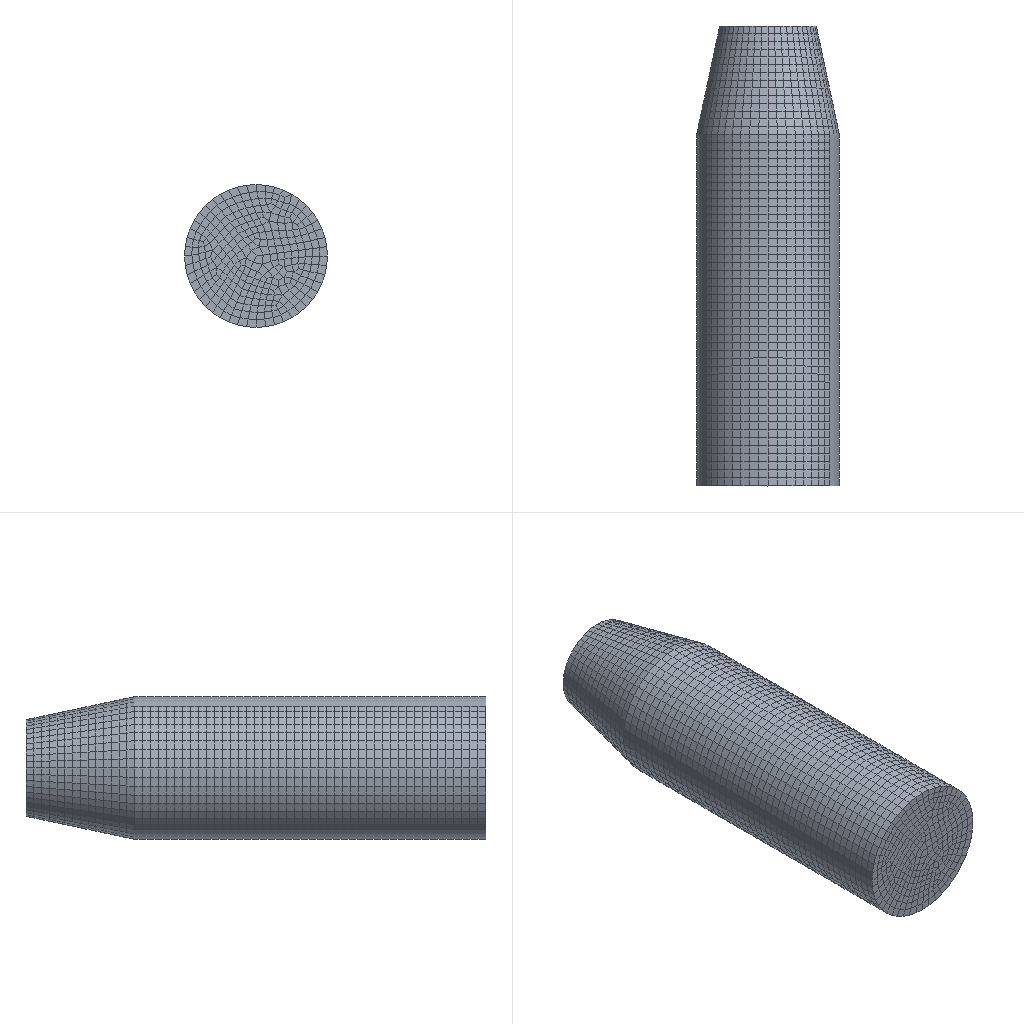Simulation study | abaqus
Set-up summary:
category,name,step,type,value,unit,region
solver,abaqus
solver,version,,,Abaqus/Explicit 3DEXPERIENCE R2017x
units,not stated in the deck,,not stated
analysis,deck,,transient,transient
load_step,Step-1,Step-1,transient
load_step,requested,,,1
mesh,nodes,,,20181
mesh,elements,,,18386
element_type,C3D8RT,,solid,18386
load,load commands in deck,,count,4
bc,support commands in deck,,count,20
material,MATERIAL-2,,in results
material,ZHAJIAN,,in results
check,setup vs results,,match,"per instance, exact: element labels, types and connectivity; labels of the nodes the elements use; coordinates of those nodes at SINGLE_PRECISION in 3 of 4 instance(s)"
Abaqus input file, long lists of numbers shortened:
*Heading
** Job name: Job-7 Model name: Job-model-Copy
** Generated by: Abaqus/CAE 2017
*Preprint, echo=NO, model=NO, history=NO, contact=NO
**
** PARTS
**
*Part, name=GUN-1
*End Part
**
*Part, name=GUN-2
*End Part
**
*Part, name=GUN-3
*End Part
**
*Part, name=ZHAJIAN
*Node
      1,        16.25,           0.,           0.
      2,           0.,           0.,           0.
** (20176 more lines like these left out)
*Element, type=C3D8RT
    1,   436,   447,   424,   454,    94,   105,    82,   112
    2,   379,   447,   436,   378,    37,   105,    94,    36
** (18384 more lines like these left out)
*Nset, nset=SET-1, generate
     1,  20178,      1
*Elset, elset=SET-1, generate
     1,  18386,      1
*Nset, nset=SET-16, generate
     1,  20178,      1
*Elset, elset=SET-16, generate
     1,  18386,      1
*Nset, nset=SET-17, generate
     1,  20178,      1
*Elset, elset=SET-17, generate
     1,  18386,      1
*Nset, nset=SET-21, generate
     1,  20178,      1
*Elset, elset=SET-21, generate
     1,  18386,      1
*Nset, nset=SET-22, generate
     1,  20178,      1
*Elset, elset=SET-22, generate
     1,  18386,      1
*Nset, nset=SET-23, generate
     1,  20178,      1
*Elset, elset=SET-23, generate
     1,  18386,      1
*Nset, nset=SET-24, generate
     1,  20178,      1
*Elset, elset=SET-24, generate
     1,  18386,      1
*Nset, nset=SET-25, generate
     1,  20178,      1
*Elset, elset=SET-25, generate
     1,  18386,      1
*Nset, nset=SET-26, generate
     1,  20178,      1
*Elset, elset=SET-26, generate
     1,  18386,      1
*Nset, nset=SET-27, generate
     1,  20178,      1
*Elset, elset=SET-27, generate
     1,  18386,      1
*Nset, nset=SET-28, generate
     1,  20178,      1
*Elset, elset=SET-28, generate
     1,  18386,      1
*Nset, nset=SET-29, generate
     1,  20178,      1
*Elset, elset=SET-29, generate
     1,  18386,      1
*Nset, nset=SET-30, generate
     1,  20178,      1
*Elset, elset=SET-30, generate
     1,  18386,      1
** Section: Section-1-SET-30
*Solid Section, elset=SET-30, material=ZHAJIAN
,
*End Part
**
**
** ASSEMBLY
**
*Assembly, name=Assembly
**
*Instance, name=GUN-1, part=GUN-1
-55.131,         110., -14.51
-55.131,         110., -14.51, -54.742, 109.611, -13.675, 159.423
*Node
      1,           0.,           0.,  -3.36777865e-15
*Nset, nset=GUN-1-RefPt_, internal
 1,
*Nset, nset=GUN-1-REFPT_, internal
 1,
*Surface, type=REVOLUTION, name=GUN-1-M_SURF-21
START,          55.,           0.
 LINE, 33.911, -30.343
 CIRCL, 31.217, -33.682, 9.277, -13.222
 LINE, 17.483, -48.41
 CIRCL, 13.826,         -50., 13.826,         -45.
 LINE,          10.,         -50.
*End Instance
**
*Instance, name=ZHAJIAN-1, part=ZHAJIAN
          0.,           0.,           0.
          0.,           0.,           0.,           0.,          -1.,           0., 7.5
*End Instance
**
*Instance, name=GUN-2, part=GUN-2
40.131,         110., -40.49
40.131,         110., -40.49, 39.596, 109.643, -39.725, 208.057
*Node
      1,           0.,           0.,  -3.36777865e-15
*Nset, nset=GUN-2-RefPt_, internal
 1,
*Nset, nset=GUN-2-REFPT_, internal
 1,
*Surface, type=REVOLUTION, name=GUN-2-M_SURF-19
START,          55.,           0.
 LINE, 33.911, -30.343
 CIRCL, 31.217, -33.682, 9.277, -13.222
 LINE, 17.483, -48.41
 CIRCL, 13.826,         -50., 13.826,         -45.
 LINE,          10.,         -50.
*End Instance
**
*Instance, name=GUN-3, part=GUN-3
         15.,         110.,          55.
         15.,         110.,          55., 15.995, 109.959, 55.087, 130.203
*Node
      1,           0.,           0.,  -3.36777865e-15
*Nset, nset=GUN-3-RefPt_, internal
 1,
*Nset, nset=GUN-3-REFPT_, internal
 1,
*Surface, type=REVOLUTION, name=GUN-3-M_SURF-27
START,          55.,           0.
 LINE, 33.911, -30.343
 CIRCL, 31.217, -33.682, 9.277, -13.222
 LINE, 17.483, -48.41
 CIRCL, 13.826,         -50., 13.826,         -45.
 LINE,          10.,         -50.
*End Instance
**
*Node
      1,           0.,    104.699,           0.
      2,           0.,           0.,           0.
*Nset, nset=M_SET-28
 1,
*Nset, nset=M_SET-42
 2,
*Nset, nset=M_SET-43
 1,
*Nset, nset=SET-30, instance=GUN-1
 1,
*Nset, nset=SET-30, instance=GUN-2
 1,
*Nset, nset=SET-31, instance=GUN-1
 1,
*Nset, nset=SET-32, instance=GUN-2
 1,
*Nset, nset=SET-34
 1,
*Nset, nset=SET-35, instance=ZHAJIAN-1, generate
     1,  20178,      1
*Elset, elset=SET-35, instance=ZHAJIAN-1, generate
     1,  18386,      1
*Nset, nset=SET-36, instance=GUN-2
 1,
*Nset, nset=SET-38, instance=GUN-1
 1,
*Nset, nset=SET-38, instance=GUN-2
 1,
*Nset, nset=SET-38, instance=GUN-3
 1,
*Nset, nset=SET-39, instance=GUN-3
 1,
*Nset, nset=SET-44
 1, 2
*Nset, nset=SET-45, instance=ZHAJIAN-1, generate
     1,  20178,      1
*Nset, nset=SET-45
 2,
*Elset, elset=SET-45, instance=ZHAJIAN-1, generate
     1,  18386,      1
*Nset, nset=SET-46, instance=GUN-2
 1,
*Nset, nset=SET-47, instance=GUN-1
 1,
*Nset, nset=SET-48, instance=GUN-2
 1,
*Nset, nset=SET-49, instance=ZHAJIAN-1, generate
     1,  20178,      1
*Nset, nset=SET-49
 2,
*Elset, elset=SET-49, instance=ZHAJIAN-1, generate
     1,  18386,      1
*Nset, nset=SET-50, instance=ZHAJIAN-1, generate
     1,  20178,      1
*Nset, nset=SET-50
 2,
*Elset, elset=SET-50, instance=ZHAJIAN-1, generate
     1,  18386,      1
*Nset, nset=SET-51, instance=GUN-1
 1,
*Nset, nset=SET-52, instance=GUN-2
 1,
*Nset, nset=SET-53, instance=GUN-3
 1,
*Nset, nset=SET-54, instance=ZHAJIAN-1
     1,     3,     4,    23,    24,    25,    26,    27,    28,    29,    30,    31,    32,    33,    34,    35
    36,    37,    38,    39,    40,    41,    42,    43,    44,    45,    46,    47,    48,    49,    50,    51
** (175 more lines like these left out)
*Elset, elset=SET-54, instance=ZHAJIAN-1
     2,    16,    18,    24,    27,    30,    31,    33,    36,    42,    45,    46,    47,    48,    50,    52
   113,   114,   120,   145,   152,   156,   169,   172,   179,   189,   199,   200,   202,   205,   208,   211
** (172 more lines like these left out)
*Nset, nset=SET-55, instance=GUN-1
 1,
*Nset, nset=SET-55, instance=GUN-2
 1,
*Nset, nset=SET-55, instance=GUN-3
 1,
*Nset, nset=SET-56, instance=GUN-3
 1,
*Nset, nset=SET-57, instance=ZHAJIAN-1, generate
     1,  20178,      1
*Nset, nset=SET-57
 2,
*Elset, elset=SET-57, instance=ZHAJIAN-1, generate
     1,  18386,      1
*Nset, nset=SET-58, instance=ZHAJIAN-1, generate
     1,  20178,      1
*Elset, elset=SET-58, instance=ZHAJIAN-1, generate
     1,  18386,      1
*Nset, nset=SET-59, instance=ZHAJIAN-1, generate
     1,  20178,      1
*Elset, elset=SET-59, instance=ZHAJIAN-1, generate
     1,  18386,      1
*Nset, nset=SET-60, instance=ZHAJIAN-1, generate
     1,  20178,      1
*Elset, elset=SET-60, instance=ZHAJIAN-1, generate
     1,  18386,      1
*Nset, nset=SET-61, instance=ZHAJIAN-1, generate
     1,  20178,      1
*Elset, elset=SET-61, instance=ZHAJIAN-1, generate
     1,  18386,      1
*Nset, nset=SET-62, instance=ZHAJIAN-1, generate
     1,  20178,      1
*Nset, nset=SET-62
 2,
*Elset, elset=SET-62, instance=ZHAJIAN-1, generate
     1,  18386,      1
*Nset, nset=SET-63, instance=ZHAJIAN-1, generate
     1,  20178,      1
*Nset, nset=SET-63
 2,
*Elset, elset=SET-63, instance=ZHAJIAN-1, generate
     1,  18386,      1
*Nset, nset=SET-64, instance=ZHAJIAN-1, generate
     1,  20178,      1
*Nset, nset=SET-64
 2,
*Elset, elset=SET-64, instance=ZHAJIAN-1, generate
     1,  18386,      1
*Nset, nset=SET-66
 1, 2
*Elset, elset=_M_SURF-38_S2, internal, instance=ZHAJIAN-1, generate
   1,  317,    1
*Elset, elset=_M_SURF-38_S3, internal, instance=ZHAJIAN-1
    30,   152,   172,   199,   200,   208,   234,   347,   469,   489,   516,   517,   525,   551,   664,   786
   806,   833,   834,   842,   868,   981,  1103,  1123,  1150,  1151,  1159,  1185,  1298,  1420,  1440,  1467
** (24 more lines like these left out)
*Elset, elset=_M_SURF-38_S4, internal, instance=ZHAJIAN-1
    16,    18,    24,    31,    42,    46,    47,    48,    50,    52,   114,   120,   189,   227,   247,   256
   261,   264,   265,   266,   333,   335,   341,   348,   359,   363,   364,   365,   367,   369,   431,   437
** (71 more lines like these left out)
*Elset, elset=_M_SURF-38_S5, internal, instance=ZHAJIAN-1
   113,   156,   430,   473,   747,   790,  1064,  1107,  1381,  1424,  1698,  1741,  2015,  2058,  2332,  2375
  2649,  2692,  2966,  3009,  3283,  3326,  3600,  3643,  3917,  3960,  4234,  4277,  4551,  4594,  4868,  4911
** (6 more lines like these left out)
*Elset, elset=_M_SURF-38_S6, internal, instance=ZHAJIAN-1
     2,    27,    33,    36,    45,   145,   169,   179,   202,   205,   211,   218,   224,   226,   233,   236
   246,   257,   260,   319,   344,   350,   353,   362,   462,   486,   496,   519,   522,   528,   535,   541
** (67 more lines like these left out)
*Elset, elset=_M_SURF-40_S2, internal, instance=ZHAJIAN-1, generate
   1,  317,    1
*Elset, elset=_M_SURF-40_S3, internal, instance=ZHAJIAN-1
    30,   152,   172,   199,   200,   208,   234,   347,   469,   489,   516,   517,   525,   551,   664,   786
   806,   833,   834,   842,   868,   981,  1103,  1123,  1150,  1151,  1159,  1185,  1298,  1420,  1440,  1467
** (24 more lines like these left out)
*Elset, elset=_M_SURF-40_S4, internal, instance=ZHAJIAN-1
    16,    18,    24,    31,    42,    46,    47,    48,    50,    52,   114,   120,   189,   227,   247,   256
   261,   264,   265,   266,   333,   335,   341,   348,   359,   363,   364,   365,   367,   369,   431,   437
** (71 more lines like these left out)
*Elset, elset=_M_SURF-40_S5, internal, instance=ZHAJIAN-1
   113,   156,   430,   473,   747,   790,  1064,  1107,  1381,  1424,  1698,  1741,  2015,  2058,  2332,  2375
  2649,  2692,  2966,  3009,  3283,  3326,  3600,  3643,  3917,  3960,  4234,  4277,  4551,  4594,  4868,  4911
** (6 more lines like these left out)
*Elset, elset=_M_SURF-40_S6, internal, instance=ZHAJIAN-1
     2,    27,    33,    36,    45,   145,   169,   179,   202,   205,   211,   218,   224,   226,   233,   236
   246,   257,   260,   319,   344,   350,   353,   362,   462,   486,   496,   519,   522,   528,   535,   541
** (67 more lines like these left out)
*Elset, elset=_M_SURF-45_S2, internal, instance=ZHAJIAN-1, generate
   1,  317,    1
*Elset, elset=_M_SURF-45_S3, internal, instance=ZHAJIAN-1
    30,   152,   172,   199,   200,   208,   234,   347,   469,   489,   516,   517,   525,   551,   664,   786
   806,   833,   834,   842,   868,   981,  1103,  1123,  1150,  1151,  1159,  1185,  1298,  1420,  1440,  1467
** (24 more lines like these left out)
*Elset, elset=_M_SURF-45_S4, internal, instance=ZHAJIAN-1
    16,    18,    24,    31,    42,    46,    47,    48,    50,    52,   114,   120,   189,   227,   247,   256
   261,   264,   265,   266,   333,   335,   341,   348,   359,   363,   364,   365,   367,   369,   431,   437
** (71 more lines like these left out)
*Elset, elset=_M_SURF-45_S5, internal, instance=ZHAJIAN-1
   113,   156,   430,   473,   747,   790,  1064,  1107,  1381,  1424,  1698,  1741,  2015,  2058,  2332,  2375
  2649,  2692,  2966,  3009,  3283,  3326,  3600,  3643,  3917,  3960,  4234,  4277,  4551,  4594,  4868,  4911
** (6 more lines like these left out)
*Elset, elset=_M_SURF-45_S6, internal, instance=ZHAJIAN-1
     2,    27,    33,    36,    45,   145,   169,   179,   202,   205,   211,   218,   224,   226,   233,   236
   246,   257,   260,   319,   344,   350,   353,   362,   462,   486,   496,   519,   522,   528,   535,   541
** (67 more lines like these left out)
*Nset, nset=_PICKEDSET234, internal, instance=ZHAJIAN-1, generate
     1,  20178,      1
*Elset, elset=_PICKEDSET234, internal, instance=ZHAJIAN-1, generate
     1,  18386,      1
*Nset, nset=_PICKEDSET266, internal, instance=ZHAJIAN-1, generate
     1,  20178,      1
*Elset, elset=_PICKEDSET266, internal, instance=ZHAJIAN-1, generate
     1,  18386,      1
*Nset, nset=_PICKEDSET273, internal, instance=ZHAJIAN-1, generate
     1,  20178,      1
*Elset, elset=_PICKEDSET273, internal, instance=ZHAJIAN-1, generate
     1,  18386,      1
*Nset, nset=_PICKEDSET317, internal, instance=ZHAJIAN-1, generate
     1,  20178,      1
*Elset, elset=_PICKEDSET317, internal, instance=ZHAJIAN-1, generate
     1,  18386,      1
*Elset, elset=_SURF-44_S2, internal, instance=ZHAJIAN-1, generate
   1,  317,    1
*Elset, elset=_SURF-44_S3, internal, instance=ZHAJIAN-1
    30,   152,   172,   199,   200,   208,   234,   347,   469,   489,   516,   517,   525,   551,   664,   786
   806,   833,   834,   842,   868,   981,  1103,  1123,  1150,  1151,  1159,  1185,  1298,  1420,  1440,  1467
** (24 more lines like these left out)
*Elset, elset=_SURF-44_S4, internal, instance=ZHAJIAN-1
    16,    18,    24,    31,    42,    46,    47,    48,    50,    52,   114,   120,   189,   227,   247,   256
   261,   264,   265,   266,   333,   335,   341,   348,   359,   363,   364,   365,   367,   369,   431,   437
** (71 more lines like these left out)
*Elset, elset=_SURF-44_S5, internal, instance=ZHAJIAN-1
   113,   156,   430,   473,   747,   790,  1064,  1107,  1381,  1424,  1698,  1741,  2015,  2058,  2332,  2375
  2649,  2692,  2966,  3009,  3283,  3326,  3600,  3643,  3917,  3960,  4234,  4277,  4551,  4594,  4868,  4911
** (6 more lines like these left out)
*Elset, elset=_SURF-44_S6, internal, instance=ZHAJIAN-1
     2,    27,    33,    36,    45,   145,   169,   179,   202,   205,   211,   218,   224,   226,   233,   236
   246,   257,   260,   319,   344,   350,   353,   362,   462,   486,   496,   519,   522,   528,   535,   541
** (67 more lines like these left out)
*Elset, elset=_S_SURF-19_S2, internal, instance=ZHAJIAN-1, generate
   1,  317,    1
*Elset, elset=_S_SURF-19_S3, internal, instance=ZHAJIAN-1
    30,   152,   172,   199,   200,   208,   234,   347,   469,   489,   516,   517,   525,   551,   664,   786
   806,   833,   834,   842,   868,   981,  1103,  1123,  1150,  1151,  1159,  1185,  1298,  1420,  1440,  1467
** (18 more lines like these left out)
*Elset, elset=_S_SURF-19_S4, internal, instance=ZHAJIAN-1
    16,    18,    24,    31,    42,    46,    47,    48,    50,    52,   114,   120,   189,   227,   247,   256
   261,   264,   265,   266,   333,   335,   341,   348,   359,   363,   364,   365,   367,   369,   431,   437
** (53 more lines like these left out)
*Elset, elset=_S_SURF-19_S5, internal, instance=ZHAJIAN-1
   113,   156,   430,   473,   747,   790,  1064,  1107,  1381,  1424,  1698,  1741,  2015,  2058,  2332,  2375
  2649,  2692,  2966,  3009,  3283,  3326,  3600,  3643,  3917,  3960,  4234,  4277,  4551,  4594,  4868,  4911
** (4 more lines like these left out)
*Elset, elset=_S_SURF-19_S6, internal, instance=ZHAJIAN-1
     2,    27,    33,    36,    45,   145,   169,   179,   202,   205,   211,   218,   224,   226,   233,   236
   246,   257,   260,   319,   344,   350,   353,   362,   462,   486,   496,   519,   522,   528,   535,   541
** (51 more lines like these left out)
*Elset, elset=_S_SURF-21_S2, internal, instance=ZHAJIAN-1, generate
   1,  317,    1
*Elset, elset=_S_SURF-21_S3, internal, instance=ZHAJIAN-1
    30,   152,   172,   199,   200,   208,   234,   347,   469,   489,   516,   517,   525,   551,   664,   786
   806,   833,   834,   842,   868,   981,  1103,  1123,  1150,  1151,  1159,  1185,  1298,  1420,  1440,  1467
** (18 more lines like these left out)
*Elset, elset=_S_SURF-21_S4, internal, instance=ZHAJIAN-1
    16,    18,    24,    31,    42,    46,    47,    48,    50,    52,   114,   120,   189,   227,   247,   256
   261,   264,   265,   266,   333,   335,   341,   348,   359,   363,   364,   365,   367,   369,   431,   437
** (53 more lines like these left out)
*Elset, elset=_S_SURF-21_S5, internal, instance=ZHAJIAN-1
   113,   156,   430,   473,   747,   790,  1064,  1107,  1381,  1424,  1698,  1741,  2015,  2058,  2332,  2375
  2649,  2692,  2966,  3009,  3283,  3326,  3600,  3643,  3917,  3960,  4234,  4277,  4551,  4594,  4868,  4911
** (4 more lines like these left out)
*Elset, elset=_S_SURF-21_S6, internal, instance=ZHAJIAN-1
     2,    27,    33,    36,    45,   145,   169,   179,   202,   205,   211,   218,   224,   226,   233,   236
   246,   257,   260,   319,   344,   350,   353,   362,   462,   486,   496,   519,   522,   528,   535,   541
** (51 more lines like these left out)
*Elset, elset=_S_SURF-23_S2, internal, instance=ZHAJIAN-1, generate
   1,  317,    1
*Elset, elset=_S_SURF-23_S3, internal, instance=ZHAJIAN-1
    30,   152,   172,   199,   200,   208,   234,   347,   469,   489,   516,   517,   525,   551,   664,   786
   806,   833,   834,   842,   868,   981,  1103,  1123,  1150,  1151,  1159,  1185,  1298,  1420,  1440,  1467
** (18 more lines like these left out)
*Elset, elset=_S_SURF-23_S4, internal, instance=ZHAJIAN-1
    16,    18,    24,    31,    42,    46,    47,    48,    50,    52,   114,   120,   189,   227,   247,   256
   261,   264,   265,   266,   333,   335,   341,   348,   359,   363,   364,   365,   367,   369,   431,   437
** (53 more lines like these left out)
*Elset, elset=_S_SURF-23_S5, internal, instance=ZHAJIAN-1
   113,   156,   430,   473,   747,   790,  1064,  1107,  1381,  1424,  1698,  1741,  2015,  2058,  2332,  2375
  2649,  2692,  2966,  3009,  3283,  3326,  3600,  3643,  3917,  3960,  4234,  4277,  4551,  4594,  4868,  4911
** (4 more lines like these left out)
*Elset, elset=_S_SURF-23_S6, internal, instance=ZHAJIAN-1
     2,    27,    33,    36,    45,   145,   169,   179,   202,   205,   211,   218,   224,   226,   233,   236
   246,   257,   260,   319,   344,   350,   353,   362,   462,   486,   496,   519,   522,   528,   535,   541
** (51 more lines like these left out)
*Elset, elset=_S_SURF-26_S2, internal, instance=ZHAJIAN-1, generate
   1,  317,    1
*Elset, elset=_S_SURF-27_S2, internal, instance=ZHAJIAN-1, generate
   1,  317,    1
*Elset, elset=_S_SURF-27_S3, internal, instance=ZHAJIAN-1
    30,   152,   172,   199,   200,   208,   234,   347,   469,   489,   516,   517,   525,   551,   664,   786
   806,   833,   834,   842,   868,   981,  1103,  1123,  1150,  1151,  1159,  1185,  1298,  1420,  1440,  1467
** (18 more lines like these left out)
*Elset, elset=_S_SURF-27_S4, internal, instance=ZHAJIAN-1
    16,    18,    24,    31,    42,    46,    47,    48,    50,    52,   114,   120,   189,   227,   247,   256
   261,   264,   265,   266,   333,   335,   341,   348,   359,   363,   364,   365,   367,   369,   431,   437
** (53 more lines like these left out)
*Elset, elset=_S_SURF-27_S5, internal, instance=ZHAJIAN-1
   113,   156,   430,   473,   747,   790,  1064,  1107,  1381,  1424,  1698,  1741,  2015,  2058,  2332,  2375
  2649,  2692,  2966,  3009,  3283,  3326,  3600,  3643,  3917,  3960,  4234,  4277,  4551,  4594,  4868,  4911
** (4 more lines like these left out)
*Elset, elset=_S_SURF-27_S6, internal, instance=ZHAJIAN-1
     2,    27,    33,    36,    45,   145,   169,   179,   202,   205,   211,   218,   224,   226,   233,   236
   246,   257,   260,   319,   344,   350,   353,   362,   462,   486,   496,   519,   522,   528,   535,   541
** (51 more lines like these left out)
*Elset, elset=_S_SURF-29_S2, internal, instance=ZHAJIAN-1, generate
   1,  317,    1
*Elset, elset=_S_SURF-30_S2, internal, instance=ZHAJIAN-1, generate
   1,  317,    1
*Elset, elset=_S_SURF-30_S3, internal, instance=ZHAJIAN-1
    30,   152,   172,   199,   200,   208,   234,   347,   469,   489,   516,   517,   525,   551,   664,   786
   806,   833,   834,   842,   868,   981,  1103,  1123,  1150,  1151,  1159,  1185,  1298,  1420,  1440,  1467
** (24 more lines like these left out)
*Elset, elset=_S_SURF-30_S4, internal, instance=ZHAJIAN-1
    16,    18,    24,    31,    42,    46,    47,    48,    50,    52,   114,   120,   189,   227,   247,   256
   261,   264,   265,   266,   333,   335,   341,   348,   359,   363,   364,   365,   367,   369,   431,   437
** (71 more lines like these left out)
*Elset, elset=_S_SURF-30_S5, internal, instance=ZHAJIAN-1
   113,   156,   430,   473,   747,   790,  1064,  1107,  1381,  1424,  1698,  1741,  2015,  2058,  2332,  2375
  2649,  2692,  2966,  3009,  3283,  3326,  3600,  3643,  3917,  3960,  4234,  4277,  4551,  4594,  4868,  4911
** (6 more lines like these left out)
*Elset, elset=_S_SURF-30_S6, internal, instance=ZHAJIAN-1
     2,    27,    33,    36,    45,   145,   169,   179,   202,   205,   211,   218,   224,   226,   233,   236
   246,   257,   260,   319,   344,   350,   353,   362,   462,   486,   496,   519,   522,   528,   535,   541
** (67 more lines like these left out)
*Elset, elset=_S_SURF-32_S2, internal, instance=ZHAJIAN-1, generate
   1,  317,    1
*Elset, elset=_S_SURF-32_S3, internal, instance=ZHAJIAN-1
    30,   152,   172,   199,   200,   208,   234,   347,   469,   489,   516,   517,   525,   551,   664,   786
   806,   833,   834,   842,   868,   981,  1103,  1123,  1150,  1151,  1159,  1185,  1298,  1420,  1440,  1467
** (24 more lines like these left out)
*Elset, elset=_S_SURF-32_S4, internal, instance=ZHAJIAN-1
    16,    18,    24,    31,    42,    46,    47,    48,    50,    52,   114,   120,   189,   227,   247,   256
   261,   264,   265,   266,   333,   335,   341,   348,   359,   363,   364,   365,   367,   369,   431,   437
** (71 more lines like these left out)
*Elset, elset=_S_SURF-32_S5, internal, instance=ZHAJIAN-1
   113,   156,   430,   473,   747,   790,  1064,  1107,  1381,  1424,  1698,  1741,  2015,  2058,  2332,  2375
  2649,  2692,  2966,  3009,  3283,  3326,  3600,  3643,  3917,  3960,  4234,  4277,  4551,  4594,  4868,  4911
** (6 more lines like these left out)
*Elset, elset=_S_SURF-32_S6, internal, instance=ZHAJIAN-1
     2,    27,    33,    36,    45,   145,   169,   179,   202,   205,   211,   218,   224,   226,   233,   236
   246,   257,   260,   319,   344,   350,   353,   362,   462,   486,   496,   519,   522,   528,   535,   541
** (67 more lines like these left out)
*Elset, elset=_S_SURF-34_S2, internal, instance=ZHAJIAN-1
   1,   2,   3,   4,   5,   6,   7,   8,   9,  10,  11,  12,  13,  14,  15,  16
  17,  18,  19,  20,  21,  22,  23,  24,  25,  26,  27,  28,  29,  30,  31,  32
** (12 more lines like these left out)
*Elset, elset=_S_SURF-34_S3, internal, instance=ZHAJIAN-1
    30,   152,   172,   199,   200,   208,   234,   347,   469,   489,   516,   517,   525,   551,   664,   786
   806,   833,   834,   842,   868,   981,  1103,  1123,  1150,  1151,  1159,  1185,  1298,  1420,  1440,  1467
** (24 more lines like these left out)
*Elset, elset=_S_SURF-34_S4, internal, instance=ZHAJIAN-1
    16,    18,    24,    31,    42,    46,    47,    48,    50,    52,   114,   120,   189,   227,   247,   256
   261,   264,   265,   266,   333,   335,   341,   348,   359,   363,   364,   365,   367,   369,   431,   437
** (71 more lines like these left out)
*Elset, elset=_S_SURF-34_S5, internal, instance=ZHAJIAN-1
   113,   156,   430,   473,   747,   790,  1064,  1107,  1381,  1424,  1698,  1741,  2015,  2058,  2332,  2375
  2649,  2692,  2966,  3009,  3283,  3326,  3600,  3643,  3917,  3960,  4234,  4277,  4551,  4594,  4868,  4911
** (6 more lines like these left out)
*Elset, elset=_S_SURF-34_S6, internal, instance=ZHAJIAN-1
     2,    27,    33,    36,    45,   145,   169,   179,   202,   205,   211,   218,   224,   226,   233,   236
   246,   257,   260,   319,   344,   350,   353,   362,   462,   486,   496,   519,   522,   528,   535,   541
** (67 more lines like these left out)
*Elset, elset=_S_SURF-36_S2, internal, instance=ZHAJIAN-1, generate
   1,  317,    1
*Elset, elset=_S_SURF-37_S1, internal, instance=ZHAJIAN-1, generate
 18070,  18386,      1
*Nset, nset="_T-Datum csys-1", internal
 1, 2
*Nset, nset="_T-Datum csys-2", internal, instance=GUN-1
 1,
*Nset, nset="_T-Datum csys-3", internal, instance=GUN-3
 1,
*Nset, nset="_T-Datum csys-4", internal, instance=GUN-2
 1,
*Elset, elset=_M_SURF-38_S2_1, internal, instance=ZHAJIAN-1, generate
   1,  317,    1
*Elset, elset=_M_SURF-38_S6_1, internal, instance=ZHAJIAN-1
     2,    27,    33,    36,    45,   145,   169,   179,   202,   205,   211,   218,   224,   226,   233,   236
   246,   257,   260,   319,   344,   350,   353,   362,   462,   486,   496,   519,   522,   528,   535,   541
** (67 more lines like these left out)
*Elset, elset=_M_SURF-38_S4_1, internal, instance=ZHAJIAN-1
    16,    18,    24,    31,    42,    46,    47,    48,    50,    52,   114,   120,   189,   227,   247,   256
   261,   264,   265,   266,   333,   335,   341,   348,   359,   363,   364,   365,   367,   369,   431,   437
** (71 more lines like these left out)
*Elset, elset=_M_SURF-38_S3_1, internal, instance=ZHAJIAN-1
    30,   152,   172,   199,   200,   208,   234,   347,   469,   489,   516,   517,   525,   551,   664,   786
   806,   833,   834,   842,   868,   981,  1103,  1123,  1150,  1151,  1159,  1185,  1298,  1420,  1440,  1467
** (24 more lines like these left out)
*Elset, elset=_M_SURF-38_S5_1, internal, instance=ZHAJIAN-1
   113,   156,   430,   473,   747,   790,  1064,  1107,  1381,  1424,  1698,  1741,  2015,  2058,  2332,  2375
  2649,  2692,  2966,  3009,  3283,  3326,  3600,  3643,  3917,  3960,  4234,  4277,  4551,  4594,  4868,  4911
** (6 more lines like these left out)
*Surface, type=ELEMENT, name=M_SURF-38
_M_SURF-38_S2_1, S2
_M_SURF-38_S6_1, S6
_M_SURF-38_S4_1, S4
_M_SURF-38_S3_1, S3
_M_SURF-38_S5_1, S5
*Elset, elset=_M_SURF-40_S2_1, internal, instance=ZHAJIAN-1, generate
   1,  317,    1
*Elset, elset=_M_SURF-40_S6_1, internal, instance=ZHAJIAN-1
     2,    27,    33,    36,    45,   145,   169,   179,   202,   205,   211,   218,   224,   226,   233,   236
   246,   257,   260,   319,   344,   350,   353,   362,   462,   486,   496,   519,   522,   528,   535,   541
** (67 more lines like these left out)
*Elset, elset=_M_SURF-40_S4_1, internal, instance=ZHAJIAN-1
    16,    18,    24,    31,    42,    46,    47,    48,    50,    52,   114,   120,   189,   227,   247,   256
   261,   264,   265,   266,   333,   335,   341,   348,   359,   363,   364,   365,   367,   369,   431,   437
** (71 more lines like these left out)
*Elset, elset=_M_SURF-40_S3_1, internal, instance=ZHAJIAN-1
    30,   152,   172,   199,   200,   208,   234,   347,   469,   489,   516,   517,   525,   551,   664,   786
   806,   833,   834,   842,   868,   981,  1103,  1123,  1150,  1151,  1159,  1185,  1298,  1420,  1440,  1467
** (24 more lines like these left out)
*Elset, elset=_M_SURF-40_S5_1, internal, instance=ZHAJIAN-1
   113,   156,   430,   473,   747,   790,  1064,  1107,  1381,  1424,  1698,  1741,  2015,  2058,  2332,  2375
  2649,  2692,  2966,  3009,  3283,  3326,  3600,  3643,  3917,  3960,  4234,  4277,  4551,  4594,  4868,  4911
** (6 more lines like these left out)
*Surface, type=ELEMENT, name=M_SURF-40
_M_SURF-40_S2_1, S2
_M_SURF-40_S6_1, S6
_M_SURF-40_S4_1, S4
_M_SURF-40_S3_1, S3
_M_SURF-40_S5_1, S5
*Elset, elset=_M_SURF-45_S2_1, internal, instance=ZHAJIAN-1, generate
   1,  317,    1
*Elset, elset=_M_SURF-45_S6_1, internal, instance=ZHAJIAN-1
     2,    27,    33,    36,    45,   145,   169,   179,   202,   205,   211,   218,   224,   226,   233,   236
   246,   257,   260,   319,   344,   350,   353,   362,   462,   486,   496,   519,   522,   528,   535,   541
** (67 more lines like these left out)
*Elset, elset=_M_SURF-45_S4_1, internal, instance=ZHAJIAN-1
    16,    18,    24,    31,    42,    46,    47,    48,    50,    52,   114,   120,   189,   227,   247,   256
   261,   264,   265,   266,   333,   335,   341,   348,   359,   363,   364,   365,   367,   369,   431,   437
** (71 more lines like these left out)
*Elset, elset=_M_SURF-45_S3_1, internal, instance=ZHAJIAN-1
    30,   152,   172,   199,   200,   208,   234,   347,   469,   489,   516,   517,   525,   551,   664,   786
   806,   833,   834,   842,   868,   981,  1103,  1123,  1150,  1151,  1159,  1185,  1298,  1420,  1440,  1467
** (24 more lines like these left out)
*Elset, elset=_M_SURF-45_S5_1, internal, instance=ZHAJIAN-1
   113,   156,   430,   473,   747,   790,  1064,  1107,  1381,  1424,  1698,  1741,  2015,  2058,  2332,  2375
  2649,  2692,  2966,  3009,  3283,  3326,  3600,  3643,  3917,  3960,  4234,  4277,  4551,  4594,  4868,  4911
** (6 more lines like these left out)
*Surface, type=ELEMENT, name=M_SURF-45
_M_SURF-45_S2_1, S2
_M_SURF-45_S6_1, S6
_M_SURF-45_S4_1, S4
_M_SURF-45_S3_1, S3
_M_SURF-45_S5_1, S5
*Elset, elset=_SURF-44_S2_1, internal, instance=ZHAJIAN-1, generate
   1,  317,    1
*Elset, elset=_SURF-44_S6_1, internal, instance=ZHAJIAN-1
     2,    27,    33,    36,    45,   145,   169,   179,   202,   205,   211,   218,   224,   226,   233,   236
   246,   257,   260,   319,   344,   350,   353,   362,   462,   486,   496,   519,   522,   528,   535,   541
** (67 more lines like these left out)
*Elset, elset=_SURF-44_S4_1, internal, instance=ZHAJIAN-1
    16,    18,    24,    31,    42,    46,    47,    48,    50,    52,   114,   120,   189,   227,   247,   256
   261,   264,   265,   266,   333,   335,   341,   348,   359,   363,   364,   365,   367,   369,   431,   437
** (71 more lines like these left out)
*Elset, elset=_SURF-44_S3_1, internal, instance=ZHAJIAN-1
    30,   152,   172,   199,   200,   208,   234,   347,   469,   489,   516,   517,   525,   551,   664,   786
   806,   833,   834,   842,   868,   981,  1103,  1123,  1150,  1151,  1159,  1185,  1298,  1420,  1440,  1467
** (24 more lines like these left out)
*Elset, elset=_SURF-44_S5_1, internal, instance=ZHAJIAN-1
   113,   156,   430,   473,   747,   790,  1064,  1107,  1381,  1424,  1698,  1741,  2015,  2058,  2332,  2375
  2649,  2692,  2966,  3009,  3283,  3326,  3600,  3643,  3917,  3960,  4234,  4277,  4551,  4594,  4868,  4911
** (6 more lines like these left out)
*Surface, type=ELEMENT, name=SURF-44
_SURF-44_S2_1, S2
_SURF-44_S6_1, S6
_SURF-44_S4_1, S4
_SURF-44_S3_1, S3
_SURF-44_S5_1, S5
*Elset, elset=_S_SURF-19_S5_1, internal, instance=ZHAJIAN-1
   113,   156,   430,   473,   747,   790,  1064,  1107,  1381,  1424,  1698,  1741,  2015,  2058,  2332,  2375
  2649,  2692,  2966,  3009,  3283,  3326,  3600,  3643,  3917,  3960,  4234,  4277,  4551,  4594,  4868,  4911
** (4 more lines like these left out)
*Elset, elset=_S_SURF-19_S4_1, internal, instance=ZHAJIAN-1
    16,    18,    24,    31,    42,    46,    47,    48,    50,    52,   114,   120,   189,   227,   247,   256
   261,   264,   265,   266,   333,   335,   341,   348,   359,   363,   364,   365,   367,   369,   431,   437
** (53 more lines like these left out)
*Elset, elset=_S_SURF-19_S6_1, internal, instance=ZHAJIAN-1
     2,    27,    33,    36,    45,   145,   169,   179,   202,   205,   211,   218,   224,   226,   233,   236
   246,   257,   260,   319,   344,   350,   353,   362,   462,   486,   496,   519,   522,   528,   535,   541
** (51 more lines like these left out)
*Elset, elset=_S_SURF-19_S2_1, internal, instance=ZHAJIAN-1, generate
   1,  317,    1
*Elset, elset=_S_SURF-19_S3_1, internal, instance=ZHAJIAN-1
    30,   152,   172,   199,   200,   208,   234,   347,   469,   489,   516,   517,   525,   551,   664,   786
   806,   833,   834,   842,   868,   981,  1103,  1123,  1150,  1151,  1159,  1185,  1298,  1420,  1440,  1467
** (18 more lines like these left out)
*Surface, type=ELEMENT, name=S_SURF-19
_S_SURF-19_S5_1, S5
_S_SURF-19_S4_1, S4
_S_SURF-19_S6_1, S6
_S_SURF-19_S2_1, S2
_S_SURF-19_S3_1, S3
*Elset, elset=_S_SURF-21_S5_1, internal, instance=ZHAJIAN-1
   113,   156,   430,   473,   747,   790,  1064,  1107,  1381,  1424,  1698,  1741,  2015,  2058,  2332,  2375
  2649,  2692,  2966,  3009,  3283,  3326,  3600,  3643,  3917,  3960,  4234,  4277,  4551,  4594,  4868,  4911
** (4 more lines like these left out)
*Elset, elset=_S_SURF-21_S4_1, internal, instance=ZHAJIAN-1
    16,    18,    24,    31,    42,    46,    47,    48,    50,    52,   114,   120,   189,   227,   247,   256
   261,   264,   265,   266,   333,   335,   341,   348,   359,   363,   364,   365,   367,   369,   431,   437
** (53 more lines like these left out)
*Elset, elset=_S_SURF-21_S6_1, internal, instance=ZHAJIAN-1
     2,    27,    33,    36,    45,   145,   169,   179,   202,   205,   211,   218,   224,   226,   233,   236
   246,   257,   260,   319,   344,   350,   353,   362,   462,   486,   496,   519,   522,   528,   535,   541
** (51 more lines like these left out)
*Elset, elset=_S_SURF-21_S2_1, internal, instance=ZHAJIAN-1, generate
   1,  317,    1
*Elset, elset=_S_SURF-21_S3_1, internal, instance=ZHAJIAN-1
    30,   152,   172,   199,   200,   208,   234,   347,   469,   489,   516,   517,   525,   551,   664,   786
   806,   833,   834,   842,   868,   981,  1103,  1123,  1150,  1151,  1159,  1185,  1298,  1420,  1440,  1467
** (18 more lines like these left out)
*Surface, type=ELEMENT, name=S_SURF-21
_S_SURF-21_S5_1, S5
_S_SURF-21_S4_1, S4
_S_SURF-21_S6_1, S6
_S_SURF-21_S2_1, S2
_S_SURF-21_S3_1, S3
*Elset, elset=_S_SURF-23_S5_1, internal, instance=ZHAJIAN-1
   113,   156,   430,   473,   747,   790,  1064,  1107,  1381,  1424,  1698,  1741,  2015,  2058,  2332,  2375
  2649,  2692,  2966,  3009,  3283,  3326,  3600,  3643,  3917,  3960,  4234,  4277,  4551,  4594,  4868,  4911
** (4 more lines like these left out)
*Elset, elset=_S_SURF-23_S4_1, internal, instance=ZHAJIAN-1
    16,    18,    24,    31,    42,    46,    47,    48,    50,    52,   114,   120,   189,   227,   247,   256
   261,   264,   265,   266,   333,   335,   341,   348,   359,   363,   364,   365,   367,   369,   431,   437
** (53 more lines like these left out)
*Elset, elset=_S_SURF-23_S6_1, internal, instance=ZHAJIAN-1
     2,    27,    33,    36,    45,   145,   169,   179,   202,   205,   211,   218,   224,   226,   233,   236
   246,   257,   260,   319,   344,   350,   353,   362,   462,   486,   496,   519,   522,   528,   535,   541
** (51 more lines like these left out)
*Elset, elset=_S_SURF-23_S2_1, internal, instance=ZHAJIAN-1, generate
   1,  317,    1
*Elset, elset=_S_SURF-23_S3_1, internal, instance=ZHAJIAN-1
    30,   152,   172,   199,   200,   208,   234,   347,   469,   489,   516,   517,   525,   551,   664,   786
   806,   833,   834,   842,   868,   981,  1103,  1123,  1150,  1151,  1159,  1185,  1298,  1420,  1440,  1467
** (18 more lines like these left out)
*Surface, type=ELEMENT, name=S_SURF-23
_S_SURF-23_S5_1, S5
_S_SURF-23_S4_1, S4
_S_SURF-23_S6_1, S6
_S_SURF-23_S2_1, S2
_S_SURF-23_S3_1, S3
*Surface, type=ELEMENT, name=S_SURF-26
_S_SURF-26_S2, S2
*Elset, elset=_S_SURF-27_S5_1, internal, instance=ZHAJIAN-1
   113,   156,   430,   473,   747,   790,  1064,  1107,  1381,  1424,  1698,  1741,  2015,  2058,  2332,  2375
  2649,  2692,  2966,  3009,  3283,  3326,  3600,  3643,  3917,  3960,  4234,  4277,  4551,  4594,  4868,  4911
** (4 more lines like these left out)
*Elset, elset=_S_SURF-27_S4_1, internal, instance=ZHAJIAN-1
    16,    18,    24,    31,    42,    46,    47,    48,    50,    52,   114,   120,   189,   227,   247,   256
   261,   264,   265,   266,   333,   335,   341,   348,   359,   363,   364,   365,   367,   369,   431,   437
** (53 more lines like these left out)
*Elset, elset=_S_SURF-27_S6_1, internal, instance=ZHAJIAN-1
     2,    27,    33,    36,    45,   145,   169,   179,   202,   205,   211,   218,   224,   226,   233,   236
   246,   257,   260,   319,   344,   350,   353,   362,   462,   486,   496,   519,   522,   528,   535,   541
** (51 more lines like these left out)
*Elset, elset=_S_SURF-27_S2_1, internal, instance=ZHAJIAN-1, generate
   1,  317,    1
*Elset, elset=_S_SURF-27_S3_1, internal, instance=ZHAJIAN-1
    30,   152,   172,   199,   200,   208,   234,   347,   469,   489,   516,   517,   525,   551,   664,   786
   806,   833,   834,   842,   868,   981,  1103,  1123,  1150,  1151,  1159,  1185,  1298,  1420,  1440,  1467
** (18 more lines like these left out)
*Surface, type=ELEMENT, name=S_SURF-27
_S_SURF-27_S5_1, S5
_S_SURF-27_S4_1, S4
_S_SURF-27_S6_1, S6
_S_SURF-27_S2_1, S2
_S_SURF-27_S3_1, S3
*Surface, type=ELEMENT, name=S_SURF-29
_S_SURF-29_S2, S2
*Elset, elset=_S_SURF-30_S2_1, internal, instance=ZHAJIAN-1, generate
   1,  317,    1
*Elset, elset=_S_SURF-30_S6_1, internal, instance=ZHAJIAN-1
     2,    27,    33,    36,    45,   145,   169,   179,   202,   205,   211,   218,   224,   226,   233,   236
   246,   257,   260,   319,   344,   350,   353,   362,   462,   486,   496,   519,   522,   528,   535,   541
** (67 more lines like these left out)
*Elset, elset=_S_SURF-30_S4_1, internal, instance=ZHAJIAN-1
    16,    18,    24,    31,    42,    46,    47,    48,    50,    52,   114,   120,   189,   227,   247,   256
   261,   264,   265,   266,   333,   335,   341,   348,   359,   363,   364,   365,   367,   369,   431,   437
** (71 more lines like these left out)
*Elset, elset=_S_SURF-30_S3_1, internal, instance=ZHAJIAN-1
    30,   152,   172,   199,   200,   208,   234,   347,   469,   489,   516,   517,   525,   551,   664,   786
   806,   833,   834,   842,   868,   981,  1103,  1123,  1150,  1151,  1159,  1185,  1298,  1420,  1440,  1467
** (24 more lines like these left out)
*Elset, elset=_S_SURF-30_S5_1, internal, instance=ZHAJIAN-1
   113,   156,   430,   473,   747,   790,  1064,  1107,  1381,  1424,  1698,  1741,  2015,  2058,  2332,  2375
  2649,  2692,  2966,  3009,  3283,  3326,  3600,  3643,  3917,  3960,  4234,  4277,  4551,  4594,  4868,  4911
** (6 more lines like these left out)
*Surface, type=ELEMENT, name=S_SURF-30
_S_SURF-30_S2_1, S2
_S_SURF-30_S6_1, S6
_S_SURF-30_S4_1, S4
_S_SURF-30_S3_1, S3
_S_SURF-30_S5_1, S5
*Elset, elset=_S_SURF-32_S2_1, internal, instance=ZHAJIAN-1, generate
   1,  317,    1
*Elset, elset=_S_SURF-32_S6_1, internal, instance=ZHAJIAN-1
     2,    27,    33,    36,    45,   145,   169,   179,   202,   205,   211,   218,   224,   226,   233,   236
   246,   257,   260,   319,   344,   350,   353,   362,   462,   486,   496,   519,   522,   528,   535,   541
** (67 more lines like these left out)
*Elset, elset=_S_SURF-32_S4_1, internal, instance=ZHAJIAN-1
    16,    18,    24,    31,    42,    46,    47,    48,    50,    52,   114,   120,   189,   227,   247,   256
   261,   264,   265,   266,   333,   335,   341,   348,   359,   363,   364,   365,   367,   369,   431,   437
** (71 more lines like these left out)
*Elset, elset=_S_SURF-32_S3_1, internal, instance=ZHAJIAN-1
    30,   152,   172,   199,   200,   208,   234,   347,   469,   489,   516,   517,   525,   551,   664,   786
   806,   833,   834,   842,   868,   981,  1103,  1123,  1150,  1151,  1159,  1185,  1298,  1420,  1440,  1467
** (24 more lines like these left out)
*Elset, elset=_S_SURF-32_S5_1, internal, instance=ZHAJIAN-1
   113,   156,   430,   473,   747,   790,  1064,  1107,  1381,  1424,  1698,  1741,  2015,  2058,  2332,  2375
  2649,  2692,  2966,  3009,  3283,  3326,  3600,  3643,  3917,  3960,  4234,  4277,  4551,  4594,  4868,  4911
** (6 more lines like these left out)
*Surface, type=ELEMENT, name=S_SURF-32
_S_SURF-32_S2_1, S2
_S_SURF-32_S6_1, S6
_S_SURF-32_S4_1, S4
_S_SURF-32_S3_1, S3
_S_SURF-32_S5_1, S5
*Elset, elset=_S_SURF-34_S2_1, internal, instance=ZHAJIAN-1
   1,   2,   3,   4,   5,   6,   7,   8,   9,  10,  11,  12,  13,  14,  15,  16
  17,  18,  19,  20,  21,  22,  23,  24,  25,  26,  27,  28,  29,  30,  31,  32
** (12 more lines like these left out)
*Elset, elset=_S_SURF-34_S6_1, internal, instance=ZHAJIAN-1
     2,    27,    33,    36,    45,   145,   169,   179,   202,   205,   211,   218,   224,   226,   233,   236
   246,   257,   260,   319,   344,   350,   353,   362,   462,   486,   496,   519,   522,   528,   535,   541
** (67 more lines like these left out)
*Elset, elset=_S_SURF-34_S4_1, internal, instance=ZHAJIAN-1
    16,    18,    24,    31,    42,    46,    47,    48,    50,    52,   114,   120,   189,   227,   247,   256
   261,   264,   265,   266,   333,   335,   341,   348,   359,   363,   364,   365,   367,   369,   431,   437
** (71 more lines like these left out)
*Elset, elset=_S_SURF-34_S3_1, internal, instance=ZHAJIAN-1
    30,   152,   172,   199,   200,   208,   234,   347,   469,   489,   516,   517,   525,   551,   664,   786
   806,   833,   834,   842,   868,   981,  1103,  1123,  1150,  1151,  1159,  1185,  1298,  1420,  1440,  1467
** (24 more lines like these left out)
*Elset, elset=_S_SURF-34_S5_1, internal, instance=ZHAJIAN-1
   113,   156,   430,   473,   747,   790,  1064,  1107,  1381,  1424,  1698,  1741,  2015,  2058,  2332,  2375
  2649,  2692,  2966,  3009,  3283,  3326,  3600,  3643,  3917,  3960,  4234,  4277,  4551,  4594,  4868,  4911
** (6 more lines like these left out)
*Surface, type=ELEMENT, name=S_SURF-34
_S_SURF-34_S2_1, S2
_S_SURF-34_S6_1, S6
_S_SURF-34_S4_1, S4
_S_SURF-34_S3_1, S3
_S_SURF-34_S5_1, S5
*Surface, type=ELEMENT, name=S_SURF-36
_S_SURF-36_S2, S2
*Surface, type=ELEMENT, name=S_SURF-37
_S_SURF-37_S1, S1
*Nset, nset="_T-Transform__T-Datum csys-1", internal
SET-66,
*Transform, nset="_T-Transform__T-Datum csys-1"
-0.3827,           0., -0.9239,           0., 1.,           0.
*Nset, nset="_T-Transform__T-Datum csys-4", internal
SET-46,
*Transform, nset="_T-Transform__T-Datum csys-4"
-0.7198, 0.6428, 0.262, -0.342,  -4.13706863211516e-09, -0.9397
*Nset, nset="_T-Transform__T-Datum csys-2", internal
SET-47,
*Transform, nset="_T-Transform__T-Datum csys-2"
0.5868, 0.6428, 0.4924, -0.6428,  -4.13706841007055e-09, 0.766
*Nset, nset="_T-Transform__T-Datum csys-3", internal
SET-56,
*Transform, nset="_T-Transform__T-Datum csys-3"
0.133, 0.6428, -0.7544, 0.9848,  -4.13706810475922e-09, 0.1736
** Constraint: CONSTRAINT-1
*Coupling, constraint name=CONSTRAINT-1, ref node=M_SET-42, surface=S_SURF-36
*Distributing, weighting method=UNIFORM
** Constraint: CONSTRAINT-2
*Coupling, constraint name=CONSTRAINT-2, ref node=M_SET-43, surface=S_SURF-37
*Distributing, weighting method=UNIFORM
** Constraint: RigidBody-1
*Rigid Body, ref node=GUN-1.GUN-1-REFPT_, analytical surface=GUN-1.GUN-1-M_SURF-21, isothermal=YES
** Constraint: RigidBody-2
*Rigid Body, ref node=GUN-2.GUN-2-REFPT_, analytical surface=GUN-2.GUN-2-M_SURF-19, isothermal=YES
** Constraint: RigidBody-3
*Rigid Body, ref node=GUN-3.GUN-3-REFPT_, analytical surface=GUN-3.GUN-3-M_SURF-27, isothermal=YES
*End Assembly
*Amplitude, name=AMP-1, definition=SMOOTH STEP
             0.,              0.,            0.02,              1.
**
** MATERIALS
**
*Material, name=MATERIAL-2
*Conductivity
401.,
*Density
 7.93e-09,
*Elastic
130000., 0.247
*Expansion
 1.654e-05,
*Inelastic Heat Fraction
         0.6,
*Plastic
    325.,   0.,  25.
    510.,  0.6,  25.
    165.,   0., 600.
    230.,  0.6, 600.
 78.009,   0.,1200.
 87.845, 0.01,1200.
 105.199, 0.02,1200.
 142.159, 0.05,1200.
 171.616,  0.1,1200.
  183.03, 0.15,1200.
 190.006,  0.2,1200.
 197.431, 0.25,1200.
 205.498,  0.3,1200.
 212.711, 0.35,1200.
 217.888,  0.4,1200.
 221.161, 0.45,1200.
 223.965,  0.5,1200.
  228.03, 0.55,1200.
 233.358,  0.6,1200.
*Specific Heat
 3.9e+08,
*Material, name=ZHAJIAN
*Conductivity
 489.2,   0.
 485.2, 200.
 480.2, 400.
 475.3, 600.
 470.8, 700.
 468.2, 800.
 462.2, 900.
 456.2,1000.
 452.2,1100.
 445.5,1200.
 442.2,1300.
*Density
 7.93e-09,
*Depvar, delete=14
     50,
*Expansion
 1.62e-05,   0.
 1.74e-05, 200.
 1.79e-05, 400.
 1.85e-05, 600.
 1.88e-05, 700.
 1.92e-05, 800.
 1.96e-05, 900.
 2.03e-05,1000.
 2.08e-05,1100.
 2.12e-05,1200.
 2.16e-05,1300.
*Inelastic Heat Fraction
         0.6,
*Specific Heat
 3e+08,
*User Material, constants=8
130000.,  0.247,   0.01,  0.005,    0.1,   450.,    0.2, 0.0001
**
** INTERACTION PROPERTIES
**
*Surface Interaction, name=FRIC050
*Friction
 0.5,
*Surface Behavior, pressure-overclosure=HARD
*Gap Conductance
52.,0.
 0.,1.
*Gap Heat Generation
0.95, 0.95
**
** PREDEFINED FIELDS
**
** Name: Field-1   Type: Temperature
*Initial Conditions, type=TEMPERATURE
SET-51, 25.
** Name: Field-2   Type: Temperature
*Initial Conditions, type=TEMPERATURE
SET-52, 25.
** Name: Field-3   Type: Temperature
*Initial Conditions, type=TEMPERATURE
SET-53, 25.
** Name: Field-4   Type: Temperature
*Initial Conditions, type=TEMPERATURE
SET-61, 1200.
** Name: IC-1   Type: Velocity
*Initial Conditions, type=ROTATING VELOCITY
SET-45, 200., 0., 30000., 0.,
0., 0., 0., 0., 10., 0.,
** ----------------------------------------------------------------
**
** STEP: Step-1
**
*Step, name=Step-1, nlgeom=YES
*Dynamic, Explicit
, 0.015
*Bulk Viscosity
0.06, 1.2
**
** BOUNDARY CONDITIONS
**
** Name: Disp-BC-1 Type: 位移/转角
*Boundary
SET-66, 1, 1
** Name: Disp-BC-2 Type: 位移/转角
*Boundary
SET-66, 3, 3
** Name: Vel-BC-1 Type: 速度/角速度
*Boundary, type=VELOCITY
SET-46, 1, 1
** Name: Vel-BC-2 Type: 速度/角速度
*Boundary, type=VELOCITY
SET-46, 2, 2
** Name: Vel-BC-3 Type: 速度/角速度
*Boundary, type=VELOCITY
SET-46, 3, 3
** Name: Vel-BC-4 Type: 速度/角速度
*Boundary, type=VELOCITY
SET-46, 4, 4, 12.56
** Name: Vel-BC-5 Type: 速度/角速度
*Boundary, type=VELOCITY
SET-46, 5, 5
** Name: Vel-BC-6 Type: 速度/角速度
*Boundary, type=VELOCITY
SET-46, 6, 6
** Name: Vel-BC-7 Type: 速度/角速度
*Boundary, type=VELOCITY
SET-47, 1, 1
** Name: Vel-BC-8 Type: 速度/角速度
*Boundary, type=VELOCITY
SET-47, 2, 2
** Name: Vel-BC-9 Type: 速度/角速度
*Boundary, type=VELOCITY
SET-47, 3, 3
** Name: Vel-BC-10 Type: 速度/角速度
*Boundary, type=VELOCITY
SET-47, 4, 4, 12.56
** Name: Vel-BC-11 Type: 速度/角速度
*Boundary, type=VELOCITY
SET-47, 5, 5
** Name: Vel-BC-12 Type: 速度/角速度
*Boundary, type=VELOCITY
SET-47, 6, 6
** Name: Vel-BC-13 Type: 速度/角速度
*Boundary, type=VELOCITY
SET-56, 1, 1
** Name: Vel-BC-14 Type: 速度/角速度
*Boundary, type=VELOCITY
SET-56, 2, 2
** Name: Vel-BC-15 Type: 速度/角速度
*Boundary, type=VELOCITY
SET-56, 3, 3
** Name: Vel-BC-16 Type: 速度/角速度
*Boundary, type=VELOCITY
SET-56, 4, 4, 12.56
** Name: Vel-BC-17 Type: 速度/角速度
*Boundary, type=VELOCITY
SET-56, 5, 5
** Name: Vel-BC-18 Type: 速度/角速度
*Boundary, type=VELOCITY
SET-56, 6, 6
*Adaptive Mesh, elset=_PICKEDSET317, controls=ADA-1, op=NEW
**
** INTERACTIONS
**
** Interaction: INT-1-1
*Contact Pair, interaction=FRIC050, mechanical constraint=PENALTY, cpset=INT-1-1
GUN-3.GUN-3-M_SURF-27, M_SURF-38
** Interaction: INT-2-1
*Contact Pair, interaction=FRIC050, mechanical constraint=PENALTY, cpset=INT-2-1
GUN-1.GUN-1-M_SURF-21, M_SURF-40
** Interaction: INT-5-1
*Contact Pair, interaction=FRIC050, mechanical constraint=PENALTY, cpset=INT-5-1
GUN-2.GUN-2-M_SURF-19, M_SURF-45
**
** OUTPUT REQUESTS
**
*Restart, write, number interval=1, time marks=NO
**
** FIELD OUTPUT: F-Output-3
**
*Output, field, number interval=50
*Contact Output
CDISP, CSTRESS
**
** FIELD OUTPUT: F-Output-1
**
*Node Output
CF, RF, RM, RT, U, V, VT
**
** FIELD OUTPUT: F-Output-2
**
*Element Output, directions=YES
DAMAGEC, DAMAGET, DMICRT, EVF, LE, PE, PEEQ, PEVAVG, S, SDEG, STATUS, TEMP
**
** HISTORY OUTPUT: H-Output-1
**
*Output, history
*Energy Output
ALLIE, ALLKE
*End Step
Results summary:
result,step,Step-1,partial,increments=67220 time=0.009566/0.015
result,analysis,,,transient
result,last_loadstep,,,1
result,primary field,,,U
result,reaction total,,FX,-2.182,model units
result,reaction total,,FY,0.0,model units
result,reaction total,,FZ,4.765,model units